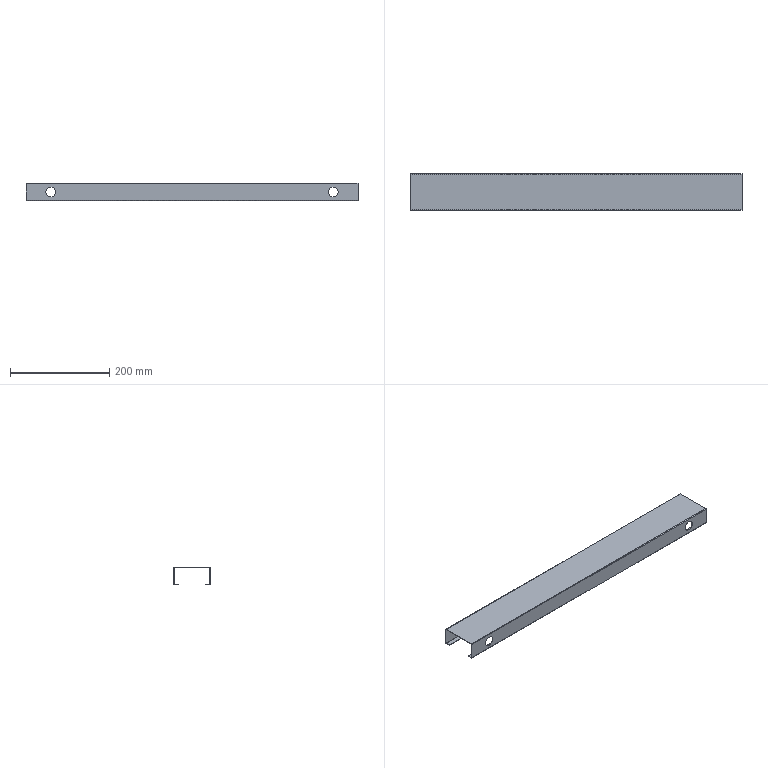Part | SolidWorks | features Cut 2, EdgeFlange 2, FlatPattern 1, ICE 1, SMBaseFlange 1, SheetMetal 1 | 1 solid | 58 faces | box 668 x 74 x 35 mm | volume 99136 mm3 | plane 40 | cylinder 18 | commonest cylinder face diameters 20 x8 0.4 x5 2.4 x5
STEP:
#1=CARTESIAN_POINT('',(-284.,36.,-27.5));
#2=VERTEX_POINT('',#1);
#3=CARTESIAN_POINT('',(-284.,36.,-7.5));
#4=VERTEX_POINT('',#3);
#5=CARTESIAN_POINT('',(-284.,36.,-17.5));
#6=DIRECTION('',(0.,1.,0.));
#7=DIRECTION('',(0.,0.,1.));
#8=AXIS2_PLACEMENT_3D('',#5,#6,#7);
#9=CIRCLE('',#8,10.);
#10=EDGE_CURVE('',#2,#4,#9,.T.);
#11=ORIENTED_EDGE('',*,*,#10,.F.);
#12=CARTESIAN_POINT('',(-284.,37.,-27.5));
#13=VERTEX_POINT('',#12);
#14=CARTESIAN_POINT('',(-284.,-37.,-27.5));
#15=DIRECTION('',(0.,1.,0.));
#16=VECTOR('',#15,1000.);
#17=LINE('',#14,#16);
#18=EDGE_CURVE('',#2,#13,#17,.T.);
#19=ORIENTED_EDGE('',*,*,#18,.T.);
#20=CARTESIAN_POINT('',(-284.,37.,-7.5));
#21=VERTEX_POINT('',#20);
#22=CARTESIAN_POINT('',(-284.,37.,-17.5));
#23=DIRECTION('',(0.,1.,0.));
#24=DIRECTION('',(0.,0.,1.));
#25=AXIS2_PLACEMENT_3D('',#22,#23,#24);
#26=CIRCLE('',#25,10.);
#27=EDGE_CURVE('',#13,#21,#26,.T.);
#28=ORIENTED_EDGE('',*,*,#27,.T.);
#29=CARTESIAN_POINT('',(-284.,-37.,-7.5));
#30=DIRECTION('',(0.,1.,0.));
#31=VECTOR('',#30,1000.);
#32=LINE('',#29,#31);
#33=EDGE_CURVE('',#4,#21,#32,.T.);
#34=ORIENTED_EDGE('',*,*,#33,.F.);
#35=EDGE_LOOP('',(#11,#19,#28,#34));
#36=FACE_OUTER_BOUND('',#35,.T.);
#37=CARTESIAN_POINT('',(-284.,-37.,-17.5));
#38=DIRECTION('',(0.,1.,0.));
#39=DIRECTION('',(0.,0.,1.));
#40=AXIS2_PLACEMENT_3D('',#37,#38,#39);
#41=CYLINDRICAL_SURFACE('',#40,10.);
#42=ADVANCED_FACE('',(#36),#41,.F.);
#43=CARTESIAN_POINT('',(284.,36.,-27.5));
#44=VERTEX_POINT('',#43);
#45=CARTESIAN_POINT('',(284.,36.,-7.5));
#46=VERTEX_POINT('',#45);
#47=CARTESIAN_POINT('',(284.,36.,-17.5));
#48=DIRECTION('',(0.,1.,0.));
#49=DIRECTION('',(0.,0.,1.));
#50=AXIS2_PLACEMENT_3D('',#47,#48,#49);
#51=CIRCLE('',#50,10.);
#52=EDGE_CURVE('',#44,#46,#51,.T.);
#53=ORIENTED_EDGE('',*,*,#52,.F.);
#54=CARTESIAN_POINT('',(284.,37.,-27.5));
#55=VERTEX_POINT('',#54);
#56=CARTESIAN_POINT('',(284.,-37.,-27.5));
#57=DIRECTION('',(0.,1.,0.));
#58=VECTOR('',#57,1000.);
#59=LINE('',#56,#58);
#60=EDGE_CURVE('',#44,#55,#59,.T.);
#61=ORIENTED_EDGE('',*,*,#60,.T.);
#62=CARTESIAN_POINT('',(284.,37.,-7.5));
#63=VERTEX_POINT('',#62);
#64=CARTESIAN_POINT('',(284.,37.,-17.5));
#65=DIRECTION('',(0.,1.,0.));
#66=DIRECTION('',(0.,0.,1.));
#67=AXIS2_PLACEMENT_3D('',#64,#65,#66);
#68=CIRCLE('',#67,10.);
#69=EDGE_CURVE('',#55,#63,#68,.T.);
#70=ORIENTED_EDGE('',*,*,#69,.T.);
#71=CARTESIAN_POINT('',(284.,-37.,-7.5));
#72=DIRECTION('',(0.,1.,0.));
#73=VECTOR('',#72,1000.);
#74=LINE('',#71,#73);
#75=EDGE_CURVE('',#46,#63,#74,.T.);
#76=ORIENTED_EDGE('',*,*,#75,.F.);
#77=EDGE_LOOP('',(#53,#61,#70,#76));
#78=FACE_OUTER_BOUND('',#77,.T.);
#79=CARTESIAN_POINT('',(284.,-37.,-17.5));
#80=DIRECTION('',(0.,1.,0.));
#81=DIRECTION('',(0.,0.,1.));
#82=AXIS2_PLACEMENT_3D('',#79,#80,#81);
#83=CYLINDRICAL_SURFACE('',#82,10.);
#84=ADVANCED_FACE('',(#78),#83,.F.);
#85=CARTESIAN_POINT('',(-284.,-37.,-27.5));
#86=VERTEX_POINT('',#85);
#87=CARTESIAN_POINT('',(-284.,-37.,-7.5));
#88=VERTEX_POINT('',#87);
#89=CARTESIAN_POINT('',(-284.,-37.,-17.5));
#90=DIRECTION('',(0.,1.,0.));
#91=DIRECTION('',(0.,0.,1.));
#92=AXIS2_PLACEMENT_3D('',#89,#90,#91);
#93=CIRCLE('',#92,10.);
#94=EDGE_CURVE('',#86,#88,#93,.T.);
#95=ORIENTED_EDGE('',*,*,#94,.F.);
#96=CARTESIAN_POINT('',(-284.,-36.,-27.5));
#97=VERTEX_POINT('',#96);
#98=CARTESIAN_POINT('',(-284.,-37.,-27.5));
#99=DIRECTION('',(0.,1.,0.));
#100=VECTOR('',#99,1000.);
#101=LINE('',#98,#100);
#102=EDGE_CURVE('',#86,#97,#101,.T.);
#103=ORIENTED_EDGE('',*,*,#102,.T.);
#104=CARTESIAN_POINT('',(-284.,-36.,-7.5));
#105=VERTEX_POINT('',#104);
#106=CARTESIAN_POINT('',(-284.,-36.,-17.5));
#107=DIRECTION('',(0.,1.,0.));
#108=DIRECTION('',(0.,0.,1.));
#109=AXIS2_PLACEMENT_3D('',#106,#107,#108);
#110=CIRCLE('',#109,10.);
#111=EDGE_CURVE('',#97,#105,#110,.T.);
#112=ORIENTED_EDGE('',*,*,#111,.T.);
#113=CARTESIAN_POINT('',(-284.,-37.,-7.5));
#114=DIRECTION('',(0.,1.,0.));
#115=VECTOR('',#114,1000.);
#116=LINE('',#113,#115);
#117=EDGE_CURVE('',#88,#105,#116,.T.);
#118=ORIENTED_EDGE('',*,*,#117,.F.);
#119=EDGE_LOOP('',(#95,#103,#112,#118));
#120=FACE_OUTER_BOUND('',#119,.T.);
#121=CARTESIAN_POINT('',(-284.,-37.,-17.5));
#122=DIRECTION('',(0.,1.,0.));
#123=DIRECTION('',(0.,0.,1.));
#124=AXIS2_PLACEMENT_3D('',#121,#122,#123);
#125=CYLINDRICAL_SURFACE('',#124,10.);
#126=ADVANCED_FACE('',(#120),#125,.F.);
#127=CARTESIAN_POINT('',(284.,-37.,-27.5));
#128=VERTEX_POINT('',#127);
#129=CARTESIAN_POINT('',(284.,-37.,-7.5));
#130=VERTEX_POINT('',#129);
#131=CARTESIAN_POINT('',(284.,-37.,-17.5));
#132=DIRECTION('',(0.,1.,0.));
#133=DIRECTION('',(0.,0.,-1.));
#134=AXIS2_PLACEMENT_3D('',#131,#132,#133);
#135=CIRCLE('',#134,10.);
#136=EDGE_CURVE('',#128,#130,#135,.T.);
#137=ORIENTED_EDGE('',*,*,#136,.F.);
#138=CARTESIAN_POINT('',(284.,-36.,-27.5));
#139=VERTEX_POINT('',#138);
#140=CARTESIAN_POINT('',(284.,-37.,-27.5));
#141=DIRECTION('',(0.,1.,0.));
#142=VECTOR('',#141,1000.);
#143=LINE('',#140,#142);
#144=EDGE_CURVE('',#128,#139,#143,.T.);
#145=ORIENTED_EDGE('',*,*,#144,.T.);
#146=CARTESIAN_POINT('',(284.,-36.,-7.5));
#147=VERTEX_POINT('',#146);
#148=CARTESIAN_POINT('',(284.,-36.,-17.5));
#149=DIRECTION('',(0.,1.,0.));
#150=DIRECTION('',(0.,0.,1.));
#151=AXIS2_PLACEMENT_3D('',#148,#149,#150);
#152=CIRCLE('',#151,10.);
#153=EDGE_CURVE('',#139,#147,#152,.T.);
#154=ORIENTED_EDGE('',*,*,#153,.T.);
#155=CARTESIAN_POINT('',(284.,-37.,-7.5));
#156=DIRECTION('',(0.,1.,0.));
#157=VECTOR('',#156,1000.);
#158=LINE('',#155,#157);
#159=EDGE_CURVE('',#130,#147,#158,.T.);
#160=ORIENTED_EDGE('',*,*,#159,.F.);
#161=EDGE_LOOP('',(#137,#145,#154,#160));
#162=FACE_OUTER_BOUND('',#161,.T.);
#163=CARTESIAN_POINT('',(284.,-37.,-17.5));
#164=DIRECTION('',(0.,1.,0.));
#165=DIRECTION('',(0.,0.,1.));
#166=AXIS2_PLACEMENT_3D('',#163,#164,#165);
#167=CYLINDRICAL_SURFACE('',#166,10.);
#168=ADVANCED_FACE('',(#162),#167,.F.);
#169=CARTESIAN_POINT('',(-152.,27.,-35.));
#170=VERTEX_POINT('',#169);
#171=CARTESIAN_POINT('',(-152.,35.8,-35.));
#172=VERTEX_POINT('',#171);
#173=CARTESIAN_POINT('',(-152.,47.,-35.));
#174=DIRECTION('',(0.,1.,0.));
#175=VECTOR('',#174,1000.);
#176=LINE('',#173,#175);
#177=EDGE_CURVE('',#170,#172,#176,.T.);
#178=ORIENTED_EDGE('',*,*,#177,.T.);
#179=CARTESIAN_POINT('',(-152.,35.8,-34.));
#180=VERTEX_POINT('',#179);
#181=CARTESIAN_POINT('',(-152.,35.8,-35.));
#182=DIRECTION('',(0.,0.,1.));
#183=VECTOR('',#182,1000.);
#184=LINE('',#181,#183);
#185=EDGE_CURVE('',#172,#180,#184,.T.);
#186=ORIENTED_EDGE('',*,*,#185,.T.);
#187=CARTESIAN_POINT('',(-152.,27.,-34.));
#188=VERTEX_POINT('',#187);
#189=CARTESIAN_POINT('',(-152.,0.,-34.));
#190=DIRECTION('',(0.,-1.,0.));
#191=VECTOR('',#190,1000.);
#192=LINE('',#189,#191);
#193=EDGE_CURVE('',#180,#188,#192,.T.);
#194=ORIENTED_EDGE('',*,*,#193,.T.);
#195=CARTESIAN_POINT('',(-152.,27.,-35.));
#196=DIRECTION('',(0.,0.,1.));
#197=VECTOR('',#196,1000.);
#198=LINE('',#195,#197);
#199=EDGE_CURVE('',#170,#188,#198,.T.);
#200=ORIENTED_EDGE('',*,*,#199,.F.);
#201=EDGE_LOOP('',(#178,#186,#194,#200));
#202=FACE_OUTER_BOUND('',#201,.T.);
#203=CARTESIAN_POINT('',(-152.,47.,-25.));
#204=DIRECTION('',(-1.,0.,0.));
#205=DIRECTION('',(0.,0.,1.));
#206=AXIS2_PLACEMENT_3D('',#203,#204,#205);
#207=PLANE('',#206);
#208=ADVANCED_FACE('',(#202),#207,.F.);
#209=CARTESIAN_POINT('',(-152.,36.,-33.8));
#210=VERTEX_POINT('',#209);
#211=CARTESIAN_POINT('',(-152.,36.,-25.));
#212=VERTEX_POINT('',#211);
#213=CARTESIAN_POINT('',(-152.,36.,0.));
#214=DIRECTION('',(0.,0.,1.));
#215=VECTOR('',#214,1000.);
#216=LINE('',#213,#215);
#217=EDGE_CURVE('',#210,#212,#216,.T.);
#218=ORIENTED_EDGE('',*,*,#217,.F.);
#219=CARTESIAN_POINT('',(-152.,37.,-33.8));
#220=VERTEX_POINT('',#219);
#221=CARTESIAN_POINT('',(-152.,36.,-33.8));
#222=DIRECTION('',(0.,1.,0.));
#223=VECTOR('',#222,1000.);
#224=LINE('',#221,#223);
#225=EDGE_CURVE('',#210,#220,#224,.T.);
#226=ORIENTED_EDGE('',*,*,#225,.T.);
#227=CARTESIAN_POINT('',(-152.,37.,-25.));
#228=VERTEX_POINT('',#227);
#229=CARTESIAN_POINT('',(-152.,37.,0.));
#230=DIRECTION('',(0.,0.,1.));
#231=VECTOR('',#230,1000.);
#232=LINE('',#229,#231);
#233=EDGE_CURVE('',#220,#228,#232,.T.);
#234=ORIENTED_EDGE('',*,*,#233,.T.);
#235=CARTESIAN_POINT('',(-152.,47.,-25.));
#236=DIRECTION('',(0.,1.,0.));
#237=VECTOR('',#236,1000.);
#238=LINE('',#235,#237);
#239=EDGE_CURVE('',#212,#228,#238,.T.);
#240=ORIENTED_EDGE('',*,*,#239,.F.);
#241=EDGE_LOOP('',(#218,#226,#234,#240));
#242=FACE_OUTER_BOUND('',#241,.T.);
#243=CARTESIAN_POINT('',(-152.,47.,-25.));
#244=DIRECTION('',(-1.,0.,0.));
#245=DIRECTION('',(0.,0.,1.));
#246=AXIS2_PLACEMENT_3D('',#243,#244,#245);
#247=PLANE('',#246);
#248=ADVANCED_FACE('',(#242),#247,.F.);
#249=CARTESIAN_POINT('',(152.,27.,-34.));
#250=VERTEX_POINT('',#249);
#251=CARTESIAN_POINT('',(152.,35.8,-34.));
#252=VERTEX_POINT('',#251);
#253=CARTESIAN_POINT('',(152.,0.,-34.));
#254=DIRECTION('',(0.,1.,0.));
#255=VECTOR('',#254,1000.);
#256=LINE('',#253,#255);
#257=EDGE_CURVE('',#250,#252,#256,.T.);
#258=ORIENTED_EDGE('',*,*,#257,.T.);
#259=CARTESIAN_POINT('',(152.,35.8,-35.));
#260=VERTEX_POINT('',#259);
#261=CARTESIAN_POINT('',(152.,35.8,-34.));
#262=DIRECTION('',(0.,0.,-1.));
#263=VECTOR('',#262,1000.);
#264=LINE('',#261,#263);
#265=EDGE_CURVE('',#252,#260,#264,.T.);
#266=ORIENTED_EDGE('',*,*,#265,.T.);
#267=CARTESIAN_POINT('',(152.,27.,-35.));
#268=VERTEX_POINT('',#267);
#269=CARTESIAN_POINT('',(152.,47.,-35.));
#270=DIRECTION('',(0.,-1.,0.));
#271=VECTOR('',#270,1000.);
#272=LINE('',#269,#271);
#273=EDGE_CURVE('',#260,#268,#272,.T.);
#274=ORIENTED_EDGE('',*,*,#273,.T.);
#275=CARTESIAN_POINT('',(152.,27.,-35.));
#276=DIRECTION('',(0.,0.,-1.));
#277=VECTOR('',#276,1000.);
#278=LINE('',#275,#277);
#279=EDGE_CURVE('',#250,#268,#278,.T.);
#280=ORIENTED_EDGE('',*,*,#279,.F.);
#281=EDGE_LOOP('',(#258,#266,#274,#280));
#282=FACE_OUTER_BOUND('',#281,.T.);
#283=CARTESIAN_POINT('',(152.,47.,-25.));
#284=DIRECTION('',(1.,0.,0.));
#285=DIRECTION('',(0.,0.,-1.));
#286=AXIS2_PLACEMENT_3D('',#283,#284,#285);
#287=PLANE('',#286);
#288=ADVANCED_FACE('',(#282),#287,.F.);
#289=CARTESIAN_POINT('',(152.,37.,-25.));
#290=VERTEX_POINT('',#289);
#291=CARTESIAN_POINT('',(152.,37.,-33.8));
#292=VERTEX_POINT('',#291);
#293=CARTESIAN_POINT('',(152.,37.,0.));
#294=DIRECTION('',(0.,0.,-1.));
#295=VECTOR('',#294,1000.);
#296=LINE('',#293,#295);
#297=EDGE_CURVE('',#290,#292,#296,.T.);
#298=ORIENTED_EDGE('',*,*,#297,.T.);
#299=CARTESIAN_POINT('',(152.,36.,-33.8));
#300=VERTEX_POINT('',#299);
#301=CARTESIAN_POINT('',(152.,37.,-33.8));
#302=DIRECTION('',(0.,-1.,0.));
#303=VECTOR('',#302,1000.);
#304=LINE('',#301,#303);
#305=EDGE_CURVE('',#292,#300,#304,.T.);
#306=ORIENTED_EDGE('',*,*,#305,.T.);
#307=CARTESIAN_POINT('',(152.,36.,-25.));
#308=VERTEX_POINT('',#307);
#309=CARTESIAN_POINT('',(152.,36.,0.));
#310=DIRECTION('',(0.,0.,-1.));
#311=VECTOR('',#310,1000.);
#312=LINE('',#309,#311);
#313=EDGE_CURVE('',#308,#300,#312,.T.);
#314=ORIENTED_EDGE('',*,*,#313,.F.);
#315=CARTESIAN_POINT('',(152.,47.,-25.));
#316=DIRECTION('',(0.,-1.,0.));
#317=VECTOR('',#316,1000.);
#318=LINE('',#315,#317);
#319=EDGE_CURVE('',#290,#308,#318,.T.);
#320=ORIENTED_EDGE('',*,*,#319,.F.);
#321=EDGE_LOOP('',(#298,#306,#314,#320));
#322=FACE_OUTER_BOUND('',#321,.T.);
#323=CARTESIAN_POINT('',(152.,47.,-25.));
#324=DIRECTION('',(1.,0.,0.));
#325=DIRECTION('',(0.,0.,-1.));
#326=AXIS2_PLACEMENT_3D('',#323,#324,#325);
#327=PLANE('',#326);
#328=ADVANCED_FACE('',(#322),#327,.F.);
#329=CARTESIAN_POINT('',(152.,35.8,-33.8));
#330=DIRECTION('',(-1.,0.,0.));
#331=DIRECTION('',(0.,0.,-1.));
#332=AXIS2_PLACEMENT_3D('',#329,#330,#331);
#333=CIRCLE('',#332,1.2);
#334=EDGE_CURVE('',#292,#260,#333,.T.);
#335=ORIENTED_EDGE('',*,*,#334,.F.);
#336=CARTESIAN_POINT('',(334.,37.,-33.8));
#337=VERTEX_POINT('',#336);
#338=CARTESIAN_POINT('',(334.,37.,-33.8));
#339=DIRECTION('',(-1.,0.,0.));
#340=VECTOR('',#339,1000.);
#341=LINE('',#338,#340);
#342=EDGE_CURVE('',#337,#292,#341,.T.);
#343=ORIENTED_EDGE('',*,*,#342,.F.);
#344=CARTESIAN_POINT('',(334.,35.8,-35.));
#345=VERTEX_POINT('',#344);
#346=CARTESIAN_POINT('',(334.,35.8,-33.8));
#347=DIRECTION('',(1.,0.,0.));
#348=DIRECTION('',(0.,0.,-1.));
#349=AXIS2_PLACEMENT_3D('',#346,#347,#348);
#350=CIRCLE('',#349,1.2);
#351=EDGE_CURVE('',#345,#337,#350,.T.);
#352=ORIENTED_EDGE('',*,*,#351,.F.);
#353=CARTESIAN_POINT('',(-334.,35.8,-35.));
#354=DIRECTION('',(-1.,0.,0.));
#355=VECTOR('',#354,1000.);
#356=LINE('',#353,#355);
#357=EDGE_CURVE('',#345,#260,#356,.T.);
#358=ORIENTED_EDGE('',*,*,#357,.T.);
#359=EDGE_LOOP('',(#335,#343,#352,#358));
#360=FACE_OUTER_BOUND('',#359,.T.);
#361=CARTESIAN_POINT('',(334.,35.8,-33.8));
#362=DIRECTION('',(1.,0.,0.));
#363=DIRECTION('',(0.,0.,-1.));
#364=AXIS2_PLACEMENT_3D('',#361,#362,#363);
#365=CYLINDRICAL_SURFACE('',#364,1.2);
#366=ADVANCED_FACE('',(#360),#365,.T.);
#367=CARTESIAN_POINT('',(334.,36.,-33.8));
#368=VERTEX_POINT('',#367);
#369=CARTESIAN_POINT('',(334.,36.,-33.8));
#370=DIRECTION('',(-1.,0.,0.));
#371=VECTOR('',#370,1000.);
#372=LINE('',#369,#371);
#373=EDGE_CURVE('',#368,#300,#372,.T.);
#374=ORIENTED_EDGE('',*,*,#373,.T.);
#375=CARTESIAN_POINT('',(152.,35.8,-33.8));
#376=DIRECTION('',(-1.,0.,0.));
#377=DIRECTION('',(0.,0.,-1.));
#378=AXIS2_PLACEMENT_3D('',#375,#376,#377);
#379=CIRCLE('',#378,0.2);
#380=EDGE_CURVE('',#300,#252,#379,.T.);
#381=ORIENTED_EDGE('',*,*,#380,.T.);
#382=CARTESIAN_POINT('',(334.,35.8,-34.));
#383=VERTEX_POINT('',#382);
#384=CARTESIAN_POINT('',(-334.,35.8,-34.));
#385=DIRECTION('',(1.,0.,0.));
#386=VECTOR('',#385,1000.);
#387=LINE('',#384,#386);
#388=EDGE_CURVE('',#252,#383,#387,.T.);
#389=ORIENTED_EDGE('',*,*,#388,.T.);
#390=CARTESIAN_POINT('',(334.,35.8,-33.8));
#391=DIRECTION('',(1.,0.,0.));
#392=DIRECTION('',(0.,0.,-1.));
#393=AXIS2_PLACEMENT_3D('',#390,#391,#392);
#394=CIRCLE('',#393,0.2);
#395=EDGE_CURVE('',#383,#368,#394,.T.);
#396=ORIENTED_EDGE('',*,*,#395,.T.);
#397=EDGE_LOOP('',(#374,#381,#389,#396));
#398=FACE_OUTER_BOUND('',#397,.T.);
#399=CARTESIAN_POINT('',(334.,35.8,-33.8));
#400=DIRECTION('',(1.,0.,0.));
#401=DIRECTION('',(0.,0.,-1.));
#402=AXIS2_PLACEMENT_3D('',#399,#400,#401);
#403=CYLINDRICAL_SURFACE('',#402,0.2);
#404=ADVANCED_FACE('',(#398),#403,.F.);
#405=CARTESIAN_POINT('',(334.,27.,-35.));
#406=VERTEX_POINT('',#405);
#407=CARTESIAN_POINT('',(0.,27.,-35.));
#408=DIRECTION('',(-1.,0.,0.));
#409=VECTOR('',#408,1000.);
#410=LINE('',#407,#409);
#411=EDGE_CURVE('',#406,#268,#410,.T.);
#412=ORIENTED_EDGE('',*,*,#411,.T.);
#413=ORIENTED_EDGE('',*,*,#273,.F.);
#414=ORIENTED_EDGE('',*,*,#357,.F.);
#415=CARTESIAN_POINT('',(334.,0.,-35.));
#416=DIRECTION('',(0.,-1.,0.));
#417=VECTOR('',#416,1000.);
#418=LINE('',#415,#417);
#419=EDGE_CURVE('',#345,#406,#418,.T.);
#420=ORIENTED_EDGE('',*,*,#419,.T.);
#421=EDGE_LOOP('',(#412,#413,#414,#420));
#422=FACE_OUTER_BOUND('',#421,.T.);
#423=CARTESIAN_POINT('',(0.,0.,-35.));
#424=DIRECTION('',(0.,0.,1.));
#425=DIRECTION('',(0.,-1.,0.));
#426=AXIS2_PLACEMENT_3D('',#423,#424,#425);
#427=PLANE('',#426);
#428=ADVANCED_FACE('',(#422),#427,.F.);
#429=ORIENTED_EDGE('',*,*,#257,.F.);
#430=CARTESIAN_POINT('',(334.,27.,-34.));
#431=VERTEX_POINT('',#430);
#432=CARTESIAN_POINT('',(-334.,27.,-34.));
#433=DIRECTION('',(-1.,0.,0.));
#434=VECTOR('',#433,1000.);
#435=LINE('',#432,#434);
#436=EDGE_CURVE('',#431,#250,#435,.T.);
#437=ORIENTED_EDGE('',*,*,#436,.F.);
#438=CARTESIAN_POINT('',(334.,27.,-34.));
#439=DIRECTION('',(0.,-1.,0.));
#440=VECTOR('',#439,1000.);
#441=LINE('',#438,#440);
#442=EDGE_CURVE('',#383,#431,#441,.T.);
#443=ORIENTED_EDGE('',*,*,#442,.F.);
#444=ORIENTED_EDGE('',*,*,#388,.F.);
#445=EDGE_LOOP('',(#429,#437,#443,#444));
#446=FACE_OUTER_BOUND('',#445,.T.);
#447=CARTESIAN_POINT('',(0.,0.,-34.));
#448=DIRECTION('',(0.,0.,1.));
#449=DIRECTION('',(0.,-1.,0.));
#450=AXIS2_PLACEMENT_3D('',#447,#448,#449);
#451=PLANE('',#450);
#452=ADVANCED_FACE('',(#446),#451,.T.);
#453=ORIENTED_EDGE('',*,*,#436,.T.);
#454=ORIENTED_EDGE('',*,*,#279,.T.);
#455=ORIENTED_EDGE('',*,*,#411,.F.);
#456=CARTESIAN_POINT('',(334.,27.,-35.));
#457=DIRECTION('',(0.,0.,1.));
#458=VECTOR('',#457,1000.);
#459=LINE('',#456,#458);
#460=EDGE_CURVE('',#406,#431,#459,.T.);
#461=ORIENTED_EDGE('',*,*,#460,.T.);
#462=EDGE_LOOP('',(#453,#454,#455,#461));
#463=FACE_OUTER_BOUND('',#462,.T.);
#464=CARTESIAN_POINT('',(-334.,27.,-35.));
#465=DIRECTION('',(0.,1.,0.));
#466=DIRECTION('',(0.,0.,1.));
#467=AXIS2_PLACEMENT_3D('',#464,#465,#466);
#468=PLANE('',#467);
#469=ADVANCED_FACE('',(#463),#468,.F.);
#470=CARTESIAN_POINT('',(334.,36.,-1.2));
#471=VERTEX_POINT('',#470);
#472=CARTESIAN_POINT('',(334.,36.,0.));
#473=DIRECTION('',(0.,0.,1.));
#474=VECTOR('',#473,1000.);
#475=LINE('',#472,#474);
#476=EDGE_CURVE('',#368,#471,#475,.T.);
#477=ORIENTED_EDGE('',*,*,#476,.F.);
#478=CARTESIAN_POINT('',(334.,36.,-33.8));
#479=DIRECTION('',(0.,1.,0.));
#480=VECTOR('',#479,1000.);
#481=LINE('',#478,#480);
#482=EDGE_CURVE('',#368,#337,#481,.T.);
#483=ORIENTED_EDGE('',*,*,#482,.T.);
#484=CARTESIAN_POINT('',(334.,37.,-1.2));
#485=VERTEX_POINT('',#484);
#486=CARTESIAN_POINT('',(334.,37.,-1.));
#487=DIRECTION('',(0.,0.,1.));
#488=VECTOR('',#487,1000.);
#489=LINE('',#486,#488);
#490=EDGE_CURVE('',#337,#485,#489,.T.);
#491=ORIENTED_EDGE('',*,*,#490,.T.);
#492=CARTESIAN_POINT('',(334.,36.,-1.2));
#493=DIRECTION('',(0.,1.,0.));
#494=VECTOR('',#493,1000.);
#495=LINE('',#492,#494);
#496=EDGE_CURVE('',#471,#485,#495,.T.);
#497=ORIENTED_EDGE('',*,*,#496,.F.);
#498=EDGE_LOOP('',(#477,#483,#491,#497));
#499=FACE_OUTER_BOUND('',#498,.T.);
#500=CARTESIAN_POINT('',(334.,37.,-1.));
#501=DIRECTION('',(1.,0.,0.));
#502=DIRECTION('',(0.,0.,-1.));
#503=AXIS2_PLACEMENT_3D('',#500,#501,#502);
#504=PLANE('',#503);
#505=ADVANCED_FACE('',(#499),#504,.T.);
#506=ORIENTED_EDGE('',*,*,#297,.F.);
#507=CARTESIAN_POINT('',(0.,37.,-25.));
#508=DIRECTION('',(1.,0.,0.));
#509=VECTOR('',#508,1000.);
#510=LINE('',#507,#509);
#511=EDGE_CURVE('',#228,#290,#510,.T.);
#512=ORIENTED_EDGE('',*,*,#511,.F.);
#513=ORIENTED_EDGE('',*,*,#233,.F.);
#514=CARTESIAN_POINT('',(-334.,37.,-33.8));
#515=VERTEX_POINT('',#514);
#516=CARTESIAN_POINT('',(334.,37.,-33.8));
#517=DIRECTION('',(-1.,0.,0.));
#518=VECTOR('',#517,1000.);
#519=LINE('',#516,#518);
#520=EDGE_CURVE('',#220,#515,#519,.T.);
#521=ORIENTED_EDGE('',*,*,#520,.T.);
#522=CARTESIAN_POINT('',(-334.,37.,-1.2));
#523=VERTEX_POINT('',#522);
#524=CARTESIAN_POINT('',(-334.,37.,-35.));
#525=DIRECTION('',(0.,0.,-1.));
#526=VECTOR('',#525,1000.);
#527=LINE('',#524,#526);
#528=EDGE_CURVE('',#523,#515,#527,.T.);
#529=ORIENTED_EDGE('',*,*,#528,.F.);
#530=CARTESIAN_POINT('',(0.,37.,-1.2));
#531=DIRECTION('',(1.,0.,0.));
#532=VECTOR('',#531,1000.);
#533=LINE('',#530,#532);
#534=EDGE_CURVE('',#523,#485,#533,.T.);
#535=ORIENTED_EDGE('',*,*,#534,.T.);
#536=ORIENTED_EDGE('',*,*,#490,.F.);
#537=ORIENTED_EDGE('',*,*,#342,.T.);
#538=EDGE_LOOP('',(#506,#512,#513,#521,#529,#535,#536,#537));
#539=FACE_OUTER_BOUND('',#538,.T.);
#540=CARTESIAN_POINT('',(-284.,37.,-17.5));
#541=DIRECTION('',(0.,1.,0.));
#542=DIRECTION('',(0.,0.,1.));
#543=AXIS2_PLACEMENT_3D('',#540,#541,#542);
#544=CIRCLE('',#543,10.);
#545=EDGE_CURVE('',#21,#13,#544,.T.);
#546=ORIENTED_EDGE('',*,*,#545,.F.);
#547=ORIENTED_EDGE('',*,*,#27,.F.);
#548=EDGE_LOOP('',(#546,#547));
#549=FACE_BOUND('',#548,.T.);
#550=CARTESIAN_POINT('',(284.,37.,-17.5));
#551=DIRECTION('',(0.,1.,0.));
#552=DIRECTION('',(0.,0.,1.));
#553=AXIS2_PLACEMENT_3D('',#550,#551,#552);
#554=CIRCLE('',#553,10.);
#555=EDGE_CURVE('',#63,#55,#554,.T.);
#556=ORIENTED_EDGE('',*,*,#555,.F.);
#557=ORIENTED_EDGE('',*,*,#69,.F.);
#558=EDGE_LOOP('',(#556,#557));
#559=FACE_BOUND('',#558,.T.);
#560=CARTESIAN_POINT('',(0.,37.,0.));
#561=DIRECTION('',(0.,1.,0.));
#562=DIRECTION('',(0.,0.,1.));
#563=AXIS2_PLACEMENT_3D('',#560,#561,#562);
#564=PLANE('',#563);
#565=ADVANCED_FACE('',(#539,#549,#559),#564,.T.);
#566=CARTESIAN_POINT('',(-284.,36.,-17.5));
#567=DIRECTION('',(0.,1.,0.));
#568=DIRECTION('',(0.,0.,1.));
#569=AXIS2_PLACEMENT_3D('',#566,#567,#568);
#570=CIRCLE('',#569,10.);
#571=EDGE_CURVE('',#4,#2,#570,.T.);
#572=ORIENTED_EDGE('',*,*,#571,.T.);
#573=ORIENTED_EDGE('',*,*,#10,.T.);
#574=EDGE_LOOP('',(#572,#573));
#575=FACE_BOUND('',#574,.T.);
#576=CARTESIAN_POINT('',(284.,36.,-17.5));
#577=DIRECTION('',(0.,1.,0.));
#578=DIRECTION('',(0.,0.,1.));
#579=AXIS2_PLACEMENT_3D('',#576,#577,#578);
#580=CIRCLE('',#579,10.);
#581=EDGE_CURVE('',#46,#44,#580,.T.);
#582=ORIENTED_EDGE('',*,*,#581,.T.);
#583=ORIENTED_EDGE('',*,*,#52,.T.);
#584=EDGE_LOOP('',(#582,#583));
#585=FACE_BOUND('',#584,.T.);
#586=CARTESIAN_POINT('',(0.,36.,-25.));
#587=DIRECTION('',(1.,0.,0.));
#588=VECTOR('',#587,1000.);
#589=LINE('',#586,#588);
#590=EDGE_CURVE('',#212,#308,#589,.T.);
#591=ORIENTED_EDGE('',*,*,#590,.T.);
#592=ORIENTED_EDGE('',*,*,#313,.T.);
#593=ORIENTED_EDGE('',*,*,#373,.F.);
#594=ORIENTED_EDGE('',*,*,#476,.T.);
#595=CARTESIAN_POINT('',(-334.,36.,-1.2));
#596=VERTEX_POINT('',#595);
#597=CARTESIAN_POINT('',(-334.,36.,-1.2));
#598=DIRECTION('',(1.,0.,0.));
#599=VECTOR('',#598,1000.);
#600=LINE('',#597,#599);
#601=EDGE_CURVE('',#596,#471,#600,.T.);
#602=ORIENTED_EDGE('',*,*,#601,.F.);
#603=CARTESIAN_POINT('',(-334.,36.,-33.8));
#604=VERTEX_POINT('',#603);
#605=CARTESIAN_POINT('',(-334.,36.,0.));
#606=DIRECTION('',(0.,0.,-1.));
#607=VECTOR('',#606,1000.);
#608=LINE('',#605,#607);
#609=EDGE_CURVE('',#596,#604,#608,.T.);
#610=ORIENTED_EDGE('',*,*,#609,.T.);
#611=CARTESIAN_POINT('',(334.,36.,-33.8));
#612=DIRECTION('',(-1.,0.,0.));
#613=VECTOR('',#612,1000.);
#614=LINE('',#611,#613);
#615=EDGE_CURVE('',#210,#604,#614,.T.);
#616=ORIENTED_EDGE('',*,*,#615,.F.);
#617=ORIENTED_EDGE('',*,*,#217,.T.);
#618=EDGE_LOOP('',(#591,#592,#593,#594,#602,#610,#616,#617));
#619=FACE_OUTER_BOUND('',#618,.T.);
#620=CARTESIAN_POINT('',(0.,36.,0.));
#621=DIRECTION('',(0.,1.,0.));
#622=DIRECTION('',(0.,0.,1.));
#623=AXIS2_PLACEMENT_3D('',#620,#621,#622);
#624=PLANE('',#623);
#625=ADVANCED_FACE('',(#575,#585,#619),#624,.F.);
#626=CARTESIAN_POINT('',(-334.,-36.,-33.8));
#627=VERTEX_POINT('',#626);
#628=CARTESIAN_POINT('',(-334.,-36.,-1.2));
#629=VERTEX_POINT('',#628);
#630=CARTESIAN_POINT('',(-334.,-36.,0.));
#631=DIRECTION('',(0.,0.,1.));
#632=VECTOR('',#631,1000.);
#633=LINE('',#630,#632);
#634=EDGE_CURVE('',#627,#629,#633,.T.);
#635=ORIENTED_EDGE('',*,*,#634,.F.);
#636=CARTESIAN_POINT('',(-334.,-37.,-33.8));
#637=VERTEX_POINT('',#636);
#638=CARTESIAN_POINT('',(-334.,-36.,-33.8));
#639=DIRECTION('',(0.,-1.,0.));
#640=VECTOR('',#639,1000.);
#641=LINE('',#638,#640);
#642=EDGE_CURVE('',#627,#637,#641,.T.);
#643=ORIENTED_EDGE('',*,*,#642,.T.);
#644=CARTESIAN_POINT('',(-334.,-37.,-1.2));
#645=VERTEX_POINT('',#644);
#646=CARTESIAN_POINT('',(-334.,-37.,-35.));
#647=DIRECTION('',(0.,0.,1.));
#648=VECTOR('',#647,1000.);
#649=LINE('',#646,#648);
#650=EDGE_CURVE('',#637,#645,#649,.T.);
#651=ORIENTED_EDGE('',*,*,#650,.T.);
#652=CARTESIAN_POINT('',(-334.,-36.,-1.2));
#653=DIRECTION('',(0.,-1.,0.));
#654=VECTOR('',#653,1000.);
#655=LINE('',#652,#654);
#656=EDGE_CURVE('',#629,#645,#655,.T.);
#657=ORIENTED_EDGE('',*,*,#656,.F.);
#658=EDGE_LOOP('',(#635,#643,#651,#657));
#659=FACE_OUTER_BOUND('',#658,.T.);
#660=CARTESIAN_POINT('',(-334.,-37.,-35.));
#661=DIRECTION('',(-1.,0.,0.));
#662=DIRECTION('',(0.,0.,1.));
#663=AXIS2_PLACEMENT_3D('',#660,#661,#662);
#664=PLANE('',#663);
#665=ADVANCED_FACE('',(#659),#664,.T.);
#666=CARTESIAN_POINT('',(-284.,-37.,-17.5));
#667=DIRECTION('',(0.,1.,0.));
#668=DIRECTION('',(0.,0.,1.));
#669=AXIS2_PLACEMENT_3D('',#666,#667,#668);
#670=CIRCLE('',#669,10.);
#671=EDGE_CURVE('',#88,#86,#670,.T.);
#672=ORIENTED_EDGE('',*,*,#671,.T.);
#673=ORIENTED_EDGE('',*,*,#94,.T.);
#674=EDGE_LOOP('',(#672,#673));
#675=FACE_BOUND('',#674,.T.);
#676=CARTESIAN_POINT('',(284.,-37.,-17.5));
#677=DIRECTION('',(0.,1.,0.));
#678=DIRECTION('',(0.,0.,-1.));
#679=AXIS2_PLACEMENT_3D('',#676,#677,#678);
#680=CIRCLE('',#679,10.);
#681=EDGE_CURVE('',#130,#128,#680,.T.);
#682=ORIENTED_EDGE('',*,*,#681,.T.);
#683=ORIENTED_EDGE('',*,*,#136,.T.);
#684=EDGE_LOOP('',(#682,#683));
#685=FACE_BOUND('',#684,.T.);
#686=CARTESIAN_POINT('',(334.,-37.,-33.8));
#687=VERTEX_POINT('',#686);
#688=CARTESIAN_POINT('',(-334.,-37.,-33.8));
#689=DIRECTION('',(1.,0.,0.));
#690=VECTOR('',#689,1000.);
#691=LINE('',#688,#690);
#692=EDGE_CURVE('',#637,#687,#691,.T.);
#693=ORIENTED_EDGE('',*,*,#692,.T.);
#694=CARTESIAN_POINT('',(334.,-37.,-1.2));
#695=VERTEX_POINT('',#694);
#696=CARTESIAN_POINT('',(334.,-37.,-1.));
#697=DIRECTION('',(0.,0.,-1.));
#698=VECTOR('',#697,1000.);
#699=LINE('',#696,#698);
#700=EDGE_CURVE('',#695,#687,#699,.T.);
#701=ORIENTED_EDGE('',*,*,#700,.F.);
#702=CARTESIAN_POINT('',(334.,-37.,-1.2));
#703=DIRECTION('',(1.,0.,0.));
#704=VECTOR('',#703,1000.);
#705=LINE('',#702,#704);
#706=EDGE_CURVE('',#645,#695,#705,.T.);
#707=ORIENTED_EDGE('',*,*,#706,.F.);
#708=ORIENTED_EDGE('',*,*,#650,.F.);
#709=EDGE_LOOP('',(#693,#701,#707,#708));
#710=FACE_OUTER_BOUND('',#709,.T.);
#711=CARTESIAN_POINT('',(0.,-37.,0.));
#712=DIRECTION('',(0.,1.,0.));
#713=DIRECTION('',(0.,0.,1.));
#714=AXIS2_PLACEMENT_3D('',#711,#712,#713);
#715=PLANE('',#714);
#716=ADVANCED_FACE('',(#675,#685,#710),#715,.F.);
#717=CARTESIAN_POINT('',(-284.,-36.,-17.5));
#718=DIRECTION('',(0.,1.,0.));
#719=DIRECTION('',(0.,0.,1.));
#720=AXIS2_PLACEMENT_3D('',#717,#718,#719);
#721=CIRCLE('',#720,10.);
#722=EDGE_CURVE('',#105,#97,#721,.T.);
#723=ORIENTED_EDGE('',*,*,#722,.F.);
#724=ORIENTED_EDGE('',*,*,#111,.F.);
#725=EDGE_LOOP('',(#723,#724));
#726=FACE_BOUND('',#725,.T.);
#727=CARTESIAN_POINT('',(284.,-36.,-17.5));
#728=DIRECTION('',(0.,1.,0.));
#729=DIRECTION('',(0.,0.,1.));
#730=AXIS2_PLACEMENT_3D('',#727,#728,#729);
#731=CIRCLE('',#730,10.);
#732=EDGE_CURVE('',#147,#139,#731,.T.);
#733=ORIENTED_EDGE('',*,*,#732,.F.);
#734=ORIENTED_EDGE('',*,*,#153,.F.);
#735=EDGE_LOOP('',(#733,#734));
#736=FACE_BOUND('',#735,.T.);
#737=CARTESIAN_POINT('',(334.,-36.,-1.2));
#738=VERTEX_POINT('',#737);
#739=CARTESIAN_POINT('',(334.,-36.,-33.8));
#740=VERTEX_POINT('',#739);
#741=CARTESIAN_POINT('',(334.,-36.,0.));
#742=DIRECTION('',(0.,0.,-1.));
#743=VECTOR('',#742,1000.);
#744=LINE('',#741,#743);
#745=EDGE_CURVE('',#738,#740,#744,.T.);
#746=ORIENTED_EDGE('',*,*,#745,.T.);
#747=CARTESIAN_POINT('',(-334.,-36.,-33.8));
#748=DIRECTION('',(1.,0.,0.));
#749=VECTOR('',#748,1000.);
#750=LINE('',#747,#749);
#751=EDGE_CURVE('',#627,#740,#750,.T.);
#752=ORIENTED_EDGE('',*,*,#751,.F.);
#753=ORIENTED_EDGE('',*,*,#634,.T.);
#754=CARTESIAN_POINT('',(334.,-36.,-1.2));
#755=DIRECTION('',(-1.,0.,0.));
#756=VECTOR('',#755,1000.);
#757=LINE('',#754,#756);
#758=EDGE_CURVE('',#738,#629,#757,.T.);
#759=ORIENTED_EDGE('',*,*,#758,.F.);
#760=EDGE_LOOP('',(#746,#752,#753,#759));
#761=FACE_OUTER_BOUND('',#760,.T.);
#762=CARTESIAN_POINT('',(0.,-36.,0.));
#763=DIRECTION('',(0.,1.,0.));
#764=DIRECTION('',(0.,0.,1.));
#765=AXIS2_PLACEMENT_3D('',#762,#763,#764);
#766=PLANE('',#765);
#767=ADVANCED_FACE('',(#726,#736,#761),#766,.T.);
#768=CARTESIAN_POINT('',(-334.,-35.8,-1.));
#769=VERTEX_POINT('',#768);
#770=CARTESIAN_POINT('',(334.,-35.8,-1.));
#771=VERTEX_POINT('',#770);
#772=CARTESIAN_POINT('',(-334.,-35.8,-1.));
#773=DIRECTION('',(1.,0.,0.));
#774=VECTOR('',#773,1000.);
#775=LINE('',#772,#774);
#776=EDGE_CURVE('',#769,#771,#775,.T.);
#777=ORIENTED_EDGE('',*,*,#776,.F.);
#778=CARTESIAN_POINT('',(-334.,35.8,-1.));
#779=VERTEX_POINT('',#778);
#780=CARTESIAN_POINT('',(-334.,37.,-1.));
#781=DIRECTION('',(0.,-1.,0.));
#782=VECTOR('',#781,1000.);
#783=LINE('',#780,#782);
#784=EDGE_CURVE('',#779,#769,#783,.T.);
#785=ORIENTED_EDGE('',*,*,#784,.F.);
#786=CARTESIAN_POINT('',(334.,35.8,-1.));
#787=VERTEX_POINT('',#786);
#788=CARTESIAN_POINT('',(334.,35.8,-1.));
#789=DIRECTION('',(-1.,0.,0.));
#790=VECTOR('',#789,1000.);
#791=LINE('',#788,#790);
#792=EDGE_CURVE('',#787,#779,#791,.T.);
#793=ORIENTED_EDGE('',*,*,#792,.F.);
#794=CARTESIAN_POINT('',(334.,37.,-1.));
#795=DIRECTION('',(0.,1.,0.));
#796=VECTOR('',#795,1000.);
#797=LINE('',#794,#796);
#798=EDGE_CURVE('',#771,#787,#797,.T.);
#799=ORIENTED_EDGE('',*,*,#798,.F.);
#800=EDGE_LOOP('',(#777,#785,#793,#799));
#801=FACE_OUTER_BOUND('',#800,.T.);
#802=CARTESIAN_POINT('',(0.,0.,-1.));
#803=DIRECTION('',(0.,0.,1.));
#804=DIRECTION('',(1.,0.,0.));
#805=AXIS2_PLACEMENT_3D('',#802,#803,#804);
#806=PLANE('',#805);
#807=ADVANCED_FACE('',(#801),#806,.F.);
#808=CARTESIAN_POINT('',(-334.,35.8,0.));
#809=VERTEX_POINT('',#808);
#810=CARTESIAN_POINT('',(-334.,-35.8,0.));
#811=VERTEX_POINT('',#810);
#812=CARTESIAN_POINT('',(-334.,37.,0.));
#813=DIRECTION('',(0.,-1.,0.));
#814=VECTOR('',#813,1000.);
#815=LINE('',#812,#814);
#816=EDGE_CURVE('',#809,#811,#815,.T.);
#817=ORIENTED_EDGE('',*,*,#816,.T.);
#818=CARTESIAN_POINT('',(334.,-35.8,0.));
#819=VERTEX_POINT('',#818);
#820=CARTESIAN_POINT('',(-334.,-35.8,0.));
#821=DIRECTION('',(1.,0.,0.));
#822=VECTOR('',#821,1000.);
#823=LINE('',#820,#822);
#824=EDGE_CURVE('',#811,#819,#823,.T.);
#825=ORIENTED_EDGE('',*,*,#824,.T.);
#826=CARTESIAN_POINT('',(334.,35.8,0.));
#827=VERTEX_POINT('',#826);
#828=CARTESIAN_POINT('',(334.,37.,0.));
#829=DIRECTION('',(0.,1.,0.));
#830=VECTOR('',#829,1000.);
#831=LINE('',#828,#830);
#832=EDGE_CURVE('',#819,#827,#831,.T.);
#833=ORIENTED_EDGE('',*,*,#832,.T.);
#834=CARTESIAN_POINT('',(334.,35.8,0.));
#835=DIRECTION('',(-1.,0.,0.));
#836=VECTOR('',#835,1000.);
#837=LINE('',#834,#836);
#838=EDGE_CURVE('',#827,#809,#837,.T.);
#839=ORIENTED_EDGE('',*,*,#838,.T.);
#840=EDGE_LOOP('',(#817,#825,#833,#839));
#841=FACE_OUTER_BOUND('',#840,.T.);
#842=CARTESIAN_POINT('',(0.,0.,0.));
#843=DIRECTION('',(0.,0.,1.));
#844=DIRECTION('',(1.,0.,0.));
#845=AXIS2_PLACEMENT_3D('',#842,#843,#844);
#846=PLANE('',#845);
#847=ADVANCED_FACE('',(#841),#846,.T.);
#848=ORIENTED_EDGE('',*,*,#784,.T.);
#849=CARTESIAN_POINT('',(-334.,-35.8,-1.));
#850=DIRECTION('',(0.,0.,1.));
#851=VECTOR('',#850,1000.);
#852=LINE('',#849,#851);
#853=EDGE_CURVE('',#769,#811,#852,.T.);
#854=ORIENTED_EDGE('',*,*,#853,.T.);
#855=ORIENTED_EDGE('',*,*,#816,.F.);
#856=CARTESIAN_POINT('',(-334.,35.8,-1.));
#857=DIRECTION('',(0.,0.,1.));
#858=VECTOR('',#857,1000.);
#859=LINE('',#856,#858);
#860=EDGE_CURVE('',#779,#809,#859,.T.);
#861=ORIENTED_EDGE('',*,*,#860,.F.);
#862=EDGE_LOOP('',(#848,#854,#855,#861));
#863=FACE_OUTER_BOUND('',#862,.T.);
#864=CARTESIAN_POINT('',(-334.,37.,-1.));
#865=DIRECTION('',(-1.,0.,0.));
#866=DIRECTION('',(0.,0.,1.));
#867=AXIS2_PLACEMENT_3D('',#864,#865,#866);
#868=PLANE('',#867);
#869=ADVANCED_FACE('',(#863),#868,.T.);
#870=CARTESIAN_POINT('',(334.,-35.8,-1.));
#871=DIRECTION('',(0.,0.,1.));
#872=VECTOR('',#871,1000.);
#873=LINE('',#870,#872);
#874=EDGE_CURVE('',#771,#819,#873,.T.);
#875=ORIENTED_EDGE('',*,*,#874,.F.);
#876=ORIENTED_EDGE('',*,*,#798,.T.);
#877=CARTESIAN_POINT('',(334.,35.8,-1.));
#878=DIRECTION('',(0.,0.,1.));
#879=VECTOR('',#878,1000.);
#880=LINE('',#877,#879);
#881=EDGE_CURVE('',#787,#827,#880,.T.);
#882=ORIENTED_EDGE('',*,*,#881,.T.);
#883=ORIENTED_EDGE('',*,*,#832,.F.);
#884=EDGE_LOOP('',(#875,#876,#882,#883));
#885=FACE_OUTER_BOUND('',#884,.T.);
#886=CARTESIAN_POINT('',(334.,37.,-1.));
#887=DIRECTION('',(1.,0.,0.));
#888=DIRECTION('',(0.,0.,-1.));
#889=AXIS2_PLACEMENT_3D('',#886,#887,#888);
#890=PLANE('',#889);
#891=ADVANCED_FACE('',(#885),#890,.T.);
#892=CARTESIAN_POINT('',(-334.,37.,-1.2));
#893=DIRECTION('',(0.,1.,0.));
#894=VECTOR('',#893,1000.);
#895=LINE('',#892,#894);
#896=EDGE_CURVE('',#596,#523,#895,.T.);
#897=ORIENTED_EDGE('',*,*,#896,.F.);
#898=CARTESIAN_POINT('',(-334.,35.8,-1.2));
#899=DIRECTION('',(-1.,0.,0.));
#900=DIRECTION('',(0.,0.,-1.));
#901=AXIS2_PLACEMENT_3D('',#898,#899,#900);
#902=CIRCLE('',#901,0.2);
#903=EDGE_CURVE('',#779,#596,#902,.T.);
#904=ORIENTED_EDGE('',*,*,#903,.F.);
#905=ORIENTED_EDGE('',*,*,#860,.T.);
#906=CARTESIAN_POINT('',(-334.,35.8,-1.2));
#907=DIRECTION('',(-1.,0.,0.));
#908=DIRECTION('',(0.,0.,-1.));
#909=AXIS2_PLACEMENT_3D('',#906,#907,#908);
#910=CIRCLE('',#909,1.2);
#911=EDGE_CURVE('',#809,#523,#910,.T.);
#912=ORIENTED_EDGE('',*,*,#911,.T.);
#913=EDGE_LOOP('',(#897,#904,#905,#912));
#914=FACE_OUTER_BOUND('',#913,.T.);
#915=CARTESIAN_POINT('',(-334.,35.8,-1.2));
#916=DIRECTION('',(-1.,0.,0.));
#917=DIRECTION('',(0.,0.,1.));
#918=AXIS2_PLACEMENT_3D('',#915,#916,#917);
#919=PLANE('',#918);
#920=ADVANCED_FACE('',(#914),#919,.T.);
#921=CARTESIAN_POINT('',(334.,35.8,-1.2));
#922=DIRECTION('',(1.,0.,0.));
#923=DIRECTION('',(0.,0.,-1.));
#924=AXIS2_PLACEMENT_3D('',#921,#922,#923);
#925=CIRCLE('',#924,0.2);
#926=EDGE_CURVE('',#471,#787,#925,.T.);
#927=ORIENTED_EDGE('',*,*,#926,.F.);
#928=ORIENTED_EDGE('',*,*,#496,.T.);
#929=CARTESIAN_POINT('',(334.,35.8,-1.2));
#930=DIRECTION('',(1.,0.,0.));
#931=DIRECTION('',(0.,0.,-1.));
#932=AXIS2_PLACEMENT_3D('',#929,#930,#931);
#933=CIRCLE('',#932,1.2);
#934=EDGE_CURVE('',#485,#827,#933,.T.);
#935=ORIENTED_EDGE('',*,*,#934,.T.);
#936=ORIENTED_EDGE('',*,*,#881,.F.);
#937=EDGE_LOOP('',(#927,#928,#935,#936));
#938=FACE_OUTER_BOUND('',#937,.T.);
#939=CARTESIAN_POINT('',(334.,35.8,-1.2));
#940=DIRECTION('',(-1.,0.,0.));
#941=DIRECTION('',(0.,0.,1.));
#942=AXIS2_PLACEMENT_3D('',#939,#940,#941);
#943=PLANE('',#942);
#944=ADVANCED_FACE('',(#938),#943,.F.);
#945=ORIENTED_EDGE('',*,*,#838,.F.);
#946=ORIENTED_EDGE('',*,*,#934,.F.);
#947=ORIENTED_EDGE('',*,*,#534,.F.);
#948=ORIENTED_EDGE('',*,*,#911,.F.);
#949=EDGE_LOOP('',(#945,#946,#947,#948));
#950=FACE_OUTER_BOUND('',#949,.T.);
#951=CARTESIAN_POINT('',(334.,35.8,-1.2));
#952=DIRECTION('',(1.,0.,0.));
#953=DIRECTION('',(0.,1.,0.));
#954=AXIS2_PLACEMENT_3D('',#951,#952,#953);
#955=CYLINDRICAL_SURFACE('',#954,1.2);
#956=ADVANCED_FACE('',(#950),#955,.T.);
#957=ORIENTED_EDGE('',*,*,#792,.T.);
#958=ORIENTED_EDGE('',*,*,#903,.T.);
#959=ORIENTED_EDGE('',*,*,#601,.T.);
#960=ORIENTED_EDGE('',*,*,#926,.T.);
#961=EDGE_LOOP('',(#957,#958,#959,#960));
#962=FACE_OUTER_BOUND('',#961,.T.);
#963=CARTESIAN_POINT('',(334.,35.8,-1.2));
#964=DIRECTION('',(1.,0.,0.));
#965=DIRECTION('',(0.,1.,0.));
#966=AXIS2_PLACEMENT_3D('',#963,#964,#965);
#967=CYLINDRICAL_SURFACE('',#966,0.2);
#968=ADVANCED_FACE('',(#962),#967,.F.);
#969=CARTESIAN_POINT('',(-334.,36.,-33.8));
#970=DIRECTION('',(0.,1.,0.));
#971=VECTOR('',#970,1000.);
#972=LINE('',#969,#971);
#973=EDGE_CURVE('',#604,#515,#972,.T.);
#974=ORIENTED_EDGE('',*,*,#973,.F.);
#975=ORIENTED_EDGE('',*,*,#609,.F.);
#976=ORIENTED_EDGE('',*,*,#896,.T.);
#977=ORIENTED_EDGE('',*,*,#528,.T.);
#978=EDGE_LOOP('',(#974,#975,#976,#977));
#979=FACE_OUTER_BOUND('',#978,.T.);
#980=CARTESIAN_POINT('',(-334.,37.,-35.));
#981=DIRECTION('',(-1.,0.,0.));
#982=DIRECTION('',(0.,0.,1.));
#983=AXIS2_PLACEMENT_3D('',#980,#981,#982);
#984=PLANE('',#983);
#985=ADVANCED_FACE('',(#979),#984,.T.);
#986=CARTESIAN_POINT('',(334.,-37.,-1.2));
#987=DIRECTION('',(0.,-1.,0.));
#988=VECTOR('',#987,1000.);
#989=LINE('',#986,#988);
#990=EDGE_CURVE('',#738,#695,#989,.T.);
#991=ORIENTED_EDGE('',*,*,#990,.F.);
#992=CARTESIAN_POINT('',(334.,-35.8,-1.2));
#993=DIRECTION('',(1.,0.,0.));
#994=DIRECTION('',(0.,0.,1.));
#995=AXIS2_PLACEMENT_3D('',#992,#993,#994);
#996=CIRCLE('',#995,0.2);
#997=EDGE_CURVE('',#771,#738,#996,.T.);
#998=ORIENTED_EDGE('',*,*,#997,.F.);
#999=ORIENTED_EDGE('',*,*,#874,.T.);
#1000=CARTESIAN_POINT('',(334.,-35.8,-1.2));
#1001=DIRECTION('',(1.,0.,0.));
#1002=DIRECTION('',(0.,0.,1.));
#1003=AXIS2_PLACEMENT_3D('',#1000,#1001,#1002);
#1004=CIRCLE('',#1003,1.2);
#1005=EDGE_CURVE('',#819,#695,#1004,.T.);
#1006=ORIENTED_EDGE('',*,*,#1005,.T.);
#1007=EDGE_LOOP('',(#991,#998,#999,#1006));
#1008=FACE_OUTER_BOUND('',#1007,.T.);
#1009=CARTESIAN_POINT('',(334.,-35.8,-1.2));
#1010=DIRECTION('',(1.,0.,0.));
#1011=DIRECTION('',(0.,0.,-1.));
#1012=AXIS2_PLACEMENT_3D('',#1009,#1010,#1011);
#1013=PLANE('',#1012);
#1014=ADVANCED_FACE('',(#1008),#1013,.T.);
#1015=CARTESIAN_POINT('',(-334.,-35.8,-1.2));
#1016=DIRECTION('',(-1.,0.,0.));
#1017=DIRECTION('',(0.,0.,1.));
#1018=AXIS2_PLACEMENT_3D('',#1015,#1016,#1017);
#1019=CIRCLE('',#1018,0.2);
#1020=EDGE_CURVE('',#629,#769,#1019,.T.);
#1021=ORIENTED_EDGE('',*,*,#1020,.F.);
#1022=ORIENTED_EDGE('',*,*,#656,.T.);
#1023=CARTESIAN_POINT('',(-334.,-35.8,-1.2));
#1024=DIRECTION('',(-1.,0.,0.));
#1025=DIRECTION('',(0.,0.,1.));
#1026=AXIS2_PLACEMENT_3D('',#1023,#1024,#1025);
#1027=CIRCLE('',#1026,1.2);
#1028=EDGE_CURVE('',#645,#811,#1027,.T.);
#1029=ORIENTED_EDGE('',*,*,#1028,.T.);
#1030=ORIENTED_EDGE('',*,*,#853,.F.);
#1031=EDGE_LOOP('',(#1021,#1022,#1029,#1030));
#1032=FACE_OUTER_BOUND('',#1031,.T.);
#1033=CARTESIAN_POINT('',(-334.,-35.8,-1.2));
#1034=DIRECTION('',(1.,0.,0.));
#1035=DIRECTION('',(0.,0.,-1.));
#1036=AXIS2_PLACEMENT_3D('',#1033,#1034,#1035);
#1037=PLANE('',#1036);
#1038=ADVANCED_FACE('',(#1032),#1037,.F.);
#1039=ORIENTED_EDGE('',*,*,#824,.F.);
#1040=ORIENTED_EDGE('',*,*,#1028,.F.);
#1041=ORIENTED_EDGE('',*,*,#706,.T.);
#1042=ORIENTED_EDGE('',*,*,#1005,.F.);
#1043=EDGE_LOOP('',(#1039,#1040,#1041,#1042));
#1044=FACE_OUTER_BOUND('',#1043,.T.);
#1045=CARTESIAN_POINT('',(-334.,-35.8,-1.2));
#1046=DIRECTION('',(-1.,0.,0.));
#1047=DIRECTION('',(0.,-1.,0.));
#1048=AXIS2_PLACEMENT_3D('',#1045,#1046,#1047);
#1049=CYLINDRICAL_SURFACE('',#1048,1.2);
#1050=ADVANCED_FACE('',(#1044),#1049,.T.);
#1051=ORIENTED_EDGE('',*,*,#776,.T.);
#1052=ORIENTED_EDGE('',*,*,#997,.T.);
#1053=ORIENTED_EDGE('',*,*,#758,.T.);
#1054=ORIENTED_EDGE('',*,*,#1020,.T.);
#1055=EDGE_LOOP('',(#1051,#1052,#1053,#1054));
#1056=FACE_OUTER_BOUND('',#1055,.T.);
#1057=CARTESIAN_POINT('',(-334.,-35.8,-1.2));
#1058=DIRECTION('',(-1.,0.,0.));
#1059=DIRECTION('',(0.,-1.,0.));
#1060=AXIS2_PLACEMENT_3D('',#1057,#1058,#1059);
#1061=CYLINDRICAL_SURFACE('',#1060,0.2);
#1062=ADVANCED_FACE('',(#1056),#1061,.F.);
#1063=CARTESIAN_POINT('',(334.,-36.,-33.8));
#1064=DIRECTION('',(0.,-1.,0.));
#1065=VECTOR('',#1064,1000.);
#1066=LINE('',#1063,#1065);
#1067=EDGE_CURVE('',#740,#687,#1066,.T.);
#1068=ORIENTED_EDGE('',*,*,#1067,.F.);
#1069=ORIENTED_EDGE('',*,*,#745,.F.);
#1070=ORIENTED_EDGE('',*,*,#990,.T.);
#1071=ORIENTED_EDGE('',*,*,#700,.T.);
#1072=EDGE_LOOP('',(#1068,#1069,#1070,#1071));
#1073=FACE_OUTER_BOUND('',#1072,.T.);
#1074=CARTESIAN_POINT('',(334.,-37.,-1.));
#1075=DIRECTION('',(1.,0.,0.));
#1076=DIRECTION('',(0.,0.,-1.));
#1077=AXIS2_PLACEMENT_3D('',#1074,#1075,#1076);
#1078=PLANE('',#1077);
#1079=ADVANCED_FACE('',(#1073),#1078,.T.);
#1080=CARTESIAN_POINT('',(334.,-35.8,-34.));
#1081=VERTEX_POINT('',#1080);
#1082=CARTESIAN_POINT('',(334.,-35.8,-35.));
#1083=VERTEX_POINT('',#1082);
#1084=CARTESIAN_POINT('',(334.,-35.8,-35.));
#1085=DIRECTION('',(0.,0.,-1.));
#1086=VECTOR('',#1085,1000.);
#1087=LINE('',#1084,#1086);
#1088=EDGE_CURVE('',#1081,#1083,#1087,.T.);
#1089=ORIENTED_EDGE('',*,*,#1088,.F.);
#1090=CARTESIAN_POINT('',(334.,-35.8,-33.8));
#1091=DIRECTION('',(1.,0.,0.));
#1092=DIRECTION('',(0.,0.,1.));
#1093=AXIS2_PLACEMENT_3D('',#1090,#1091,#1092);
#1094=CIRCLE('',#1093,0.2);
#1095=EDGE_CURVE('',#740,#1081,#1094,.T.);
#1096=ORIENTED_EDGE('',*,*,#1095,.F.);
#1097=ORIENTED_EDGE('',*,*,#1067,.T.);
#1098=CARTESIAN_POINT('',(334.,-35.8,-33.8));
#1099=DIRECTION('',(1.,0.,0.));
#1100=DIRECTION('',(0.,0.,1.));
#1101=AXIS2_PLACEMENT_3D('',#1098,#1099,#1100);
#1102=CIRCLE('',#1101,1.2);
#1103=EDGE_CURVE('',#687,#1083,#1102,.T.);
#1104=ORIENTED_EDGE('',*,*,#1103,.T.);
#1105=EDGE_LOOP('',(#1089,#1096,#1097,#1104));
#1106=FACE_OUTER_BOUND('',#1105,.T.);
#1107=CARTESIAN_POINT('',(334.,-35.8,-33.8));
#1108=DIRECTION('',(1.,0.,0.));
#1109=DIRECTION('',(0.,0.,-1.));
#1110=AXIS2_PLACEMENT_3D('',#1107,#1108,#1109);
#1111=PLANE('',#1110);
#1112=ADVANCED_FACE('',(#1106),#1111,.T.);
#1113=CARTESIAN_POINT('',(-334.,-35.8,-34.));
#1114=VERTEX_POINT('',#1113);
#1115=CARTESIAN_POINT('',(-334.,-35.8,-33.8));
#1116=DIRECTION('',(-1.,0.,0.));
#1117=DIRECTION('',(0.,0.,1.));
#1118=AXIS2_PLACEMENT_3D('',#1115,#1116,#1117);
#1119=CIRCLE('',#1118,0.2);
#1120=EDGE_CURVE('',#1114,#627,#1119,.T.);
#1121=ORIENTED_EDGE('',*,*,#1120,.F.);
#1122=CARTESIAN_POINT('',(-334.,-35.8,-35.));
#1123=VERTEX_POINT('',#1122);
#1124=CARTESIAN_POINT('',(-334.,-35.8,-34.));
#1125=DIRECTION('',(0.,0.,-1.));
#1126=VECTOR('',#1125,1000.);
#1127=LINE('',#1124,#1126);
#1128=EDGE_CURVE('',#1114,#1123,#1127,.T.);
#1129=ORIENTED_EDGE('',*,*,#1128,.T.);
#1130=CARTESIAN_POINT('',(-334.,-35.8,-33.8));
#1131=DIRECTION('',(-1.,0.,0.));
#1132=DIRECTION('',(0.,0.,1.));
#1133=AXIS2_PLACEMENT_3D('',#1130,#1131,#1132);
#1134=CIRCLE('',#1133,1.2);
#1135=EDGE_CURVE('',#1123,#637,#1134,.T.);
#1136=ORIENTED_EDGE('',*,*,#1135,.T.);
#1137=ORIENTED_EDGE('',*,*,#642,.F.);
#1138=EDGE_LOOP('',(#1121,#1129,#1136,#1137));
#1139=FACE_OUTER_BOUND('',#1138,.T.);
#1140=CARTESIAN_POINT('',(-334.,-35.8,-33.8));
#1141=DIRECTION('',(1.,0.,0.));
#1142=DIRECTION('',(0.,0.,-1.));
#1143=AXIS2_PLACEMENT_3D('',#1140,#1141,#1142);
#1144=PLANE('',#1143);
#1145=ADVANCED_FACE('',(#1139),#1144,.F.);
#1146=ORIENTED_EDGE('',*,*,#692,.F.);
#1147=ORIENTED_EDGE('',*,*,#1135,.F.);
#1148=CARTESIAN_POINT('',(334.,-35.8,-35.));
#1149=DIRECTION('',(1.,0.,0.));
#1150=VECTOR('',#1149,1000.);
#1151=LINE('',#1148,#1150);
#1152=EDGE_CURVE('',#1123,#1083,#1151,.T.);
#1153=ORIENTED_EDGE('',*,*,#1152,.T.);
#1154=ORIENTED_EDGE('',*,*,#1103,.F.);
#1155=EDGE_LOOP('',(#1146,#1147,#1153,#1154));
#1156=FACE_OUTER_BOUND('',#1155,.T.);
#1157=CARTESIAN_POINT('',(-334.,-35.8,-33.8));
#1158=DIRECTION('',(-1.,0.,0.));
#1159=DIRECTION('',(0.,0.,-1.));
#1160=AXIS2_PLACEMENT_3D('',#1157,#1158,#1159);
#1161=CYLINDRICAL_SURFACE('',#1160,1.2);
#1162=ADVANCED_FACE('',(#1156),#1161,.T.);
#1163=ORIENTED_EDGE('',*,*,#751,.T.);
#1164=ORIENTED_EDGE('',*,*,#1095,.T.);
#1165=CARTESIAN_POINT('',(334.,-35.8,-34.));
#1166=DIRECTION('',(-1.,0.,0.));
#1167=VECTOR('',#1166,1000.);
#1168=LINE('',#1165,#1167);
#1169=EDGE_CURVE('',#1081,#1114,#1168,.T.);
#1170=ORIENTED_EDGE('',*,*,#1169,.T.);
#1171=ORIENTED_EDGE('',*,*,#1120,.T.);
#1172=EDGE_LOOP('',(#1163,#1164,#1170,#1171));
#1173=FACE_OUTER_BOUND('',#1172,.T.);
#1174=CARTESIAN_POINT('',(-334.,-35.8,-33.8));
#1175=DIRECTION('',(-1.,0.,0.));
#1176=DIRECTION('',(0.,0.,-1.));
#1177=AXIS2_PLACEMENT_3D('',#1174,#1175,#1176);
#1178=CYLINDRICAL_SURFACE('',#1177,0.2);
#1179=ADVANCED_FACE('',(#1173),#1178,.F.);
#1180=ORIENTED_EDGE('',*,*,#1088,.T.);
#1181=CARTESIAN_POINT('',(334.,-27.,-35.));
#1182=VERTEX_POINT('',#1181);
#1183=CARTESIAN_POINT('',(334.,0.,-35.));
#1184=DIRECTION('',(0.,-1.,0.));
#1185=VECTOR('',#1184,1000.);
#1186=LINE('',#1183,#1185);
#1187=EDGE_CURVE('',#1182,#1083,#1186,.T.);
#1188=ORIENTED_EDGE('',*,*,#1187,.F.);
#1189=CARTESIAN_POINT('',(334.,-27.,-34.));
#1190=VERTEX_POINT('',#1189);
#1191=CARTESIAN_POINT('',(334.,-27.,-35.));
#1192=DIRECTION('',(0.,0.,1.));
#1193=VECTOR('',#1192,1000.);
#1194=LINE('',#1191,#1193);
#1195=EDGE_CURVE('',#1182,#1190,#1194,.T.);
#1196=ORIENTED_EDGE('',*,*,#1195,.T.);
#1197=CARTESIAN_POINT('',(334.,-36.,-34.));
#1198=DIRECTION('',(0.,-1.,0.));
#1199=VECTOR('',#1198,1000.);
#1200=LINE('',#1197,#1199);
#1201=EDGE_CURVE('',#1190,#1081,#1200,.T.);
#1202=ORIENTED_EDGE('',*,*,#1201,.T.);
#1203=EDGE_LOOP('',(#1180,#1188,#1196,#1202));
#1204=FACE_OUTER_BOUND('',#1203,.T.);
#1205=CARTESIAN_POINT('',(334.,-36.,-35.));
#1206=DIRECTION('',(-1.,0.,0.));
#1207=DIRECTION('',(0.,0.,1.));
#1208=AXIS2_PLACEMENT_3D('',#1205,#1206,#1207);
#1209=PLANE('',#1208);
#1210=ADVANCED_FACE('',(#1204),#1209,.F.);
#1211=ORIENTED_EDGE('',*,*,#1128,.F.);
#1212=CARTESIAN_POINT('',(-334.,-27.,-34.));
#1213=VERTEX_POINT('',#1212);
#1214=CARTESIAN_POINT('',(-334.,-27.,-34.));
#1215=DIRECTION('',(0.,1.,0.));
#1216=VECTOR('',#1215,1000.);
#1217=LINE('',#1214,#1216);
#1218=EDGE_CURVE('',#1114,#1213,#1217,.T.);
#1219=ORIENTED_EDGE('',*,*,#1218,.T.);
#1220=CARTESIAN_POINT('',(-334.,-27.,-35.));
#1221=VERTEX_POINT('',#1220);
#1222=CARTESIAN_POINT('',(-334.,-27.,-35.));
#1223=DIRECTION('',(0.,0.,1.));
#1224=VECTOR('',#1223,1000.);
#1225=LINE('',#1222,#1224);
#1226=EDGE_CURVE('',#1221,#1213,#1225,.T.);
#1227=ORIENTED_EDGE('',*,*,#1226,.F.);
#1228=CARTESIAN_POINT('',(-334.,0.,-35.));
#1229=DIRECTION('',(0.,1.,0.));
#1230=VECTOR('',#1229,1000.);
#1231=LINE('',#1228,#1230);
#1232=EDGE_CURVE('',#1123,#1221,#1231,.T.);
#1233=ORIENTED_EDGE('',*,*,#1232,.F.);
#1234=EDGE_LOOP('',(#1211,#1219,#1227,#1233));
#1235=FACE_OUTER_BOUND('',#1234,.T.);
#1236=CARTESIAN_POINT('',(-334.,-27.,-35.));
#1237=DIRECTION('',(1.,0.,0.));
#1238=DIRECTION('',(0.,0.,-1.));
#1239=AXIS2_PLACEMENT_3D('',#1236,#1237,#1238);
#1240=PLANE('',#1239);
#1241=ADVANCED_FACE('',(#1235),#1240,.F.);
#1242=ORIENTED_EDGE('',*,*,#1152,.F.);
#1243=ORIENTED_EDGE('',*,*,#1232,.T.);
#1244=CARTESIAN_POINT('',(0.,-27.,-35.));
#1245=DIRECTION('',(1.,0.,0.));
#1246=VECTOR('',#1245,1000.);
#1247=LINE('',#1244,#1246);
#1248=EDGE_CURVE('',#1221,#1182,#1247,.T.);
#1249=ORIENTED_EDGE('',*,*,#1248,.T.);
#1250=ORIENTED_EDGE('',*,*,#1187,.T.);
#1251=EDGE_LOOP('',(#1242,#1243,#1249,#1250));
#1252=FACE_OUTER_BOUND('',#1251,.T.);
#1253=CARTESIAN_POINT('',(0.,0.,-35.));
#1254=DIRECTION('',(0.,0.,1.));
#1255=DIRECTION('',(0.,-1.,0.));
#1256=AXIS2_PLACEMENT_3D('',#1253,#1254,#1255);
#1257=PLANE('',#1256);
#1258=ADVANCED_FACE('',(#1252),#1257,.F.);
#1259=ORIENTED_EDGE('',*,*,#1218,.F.);
#1260=ORIENTED_EDGE('',*,*,#1169,.F.);
#1261=ORIENTED_EDGE('',*,*,#1201,.F.);
#1262=CARTESIAN_POINT('',(334.,-27.,-34.));
#1263=DIRECTION('',(1.,0.,0.));
#1264=VECTOR('',#1263,1000.);
#1265=LINE('',#1262,#1264);
#1266=EDGE_CURVE('',#1213,#1190,#1265,.T.);
#1267=ORIENTED_EDGE('',*,*,#1266,.F.);
#1268=EDGE_LOOP('',(#1259,#1260,#1261,#1267));
#1269=FACE_OUTER_BOUND('',#1268,.T.);
#1270=CARTESIAN_POINT('',(0.,0.,-34.));
#1271=DIRECTION('',(0.,0.,1.));
#1272=DIRECTION('',(0.,-1.,0.));
#1273=AXIS2_PLACEMENT_3D('',#1270,#1271,#1272);
#1274=PLANE('',#1273);
#1275=ADVANCED_FACE('',(#1269),#1274,.T.);
#1276=ORIENTED_EDGE('',*,*,#1266,.T.);
#1277=ORIENTED_EDGE('',*,*,#1195,.F.);
#1278=ORIENTED_EDGE('',*,*,#1248,.F.);
#1279=ORIENTED_EDGE('',*,*,#1226,.T.);
#1280=EDGE_LOOP('',(#1276,#1277,#1278,#1279));
#1281=FACE_OUTER_BOUND('',#1280,.T.);
#1282=CARTESIAN_POINT('',(334.,-27.,-35.));
#1283=DIRECTION('',(0.,-1.,0.));
#1284=DIRECTION('',(0.,0.,-1.));
#1285=AXIS2_PLACEMENT_3D('',#1282,#1283,#1284);
#1286=PLANE('',#1285);
#1287=ADVANCED_FACE('',(#1281),#1286,.F.);
#1288=CARTESIAN_POINT('',(-334.,35.8,-34.));
#1289=VERTEX_POINT('',#1288);
#1290=CARTESIAN_POINT('',(-334.,35.8,-35.));
#1291=VERTEX_POINT('',#1290);
#1292=CARTESIAN_POINT('',(-334.,35.8,-35.));
#1293=DIRECTION('',(0.,0.,-1.));
#1294=VECTOR('',#1293,1000.);
#1295=LINE('',#1292,#1294);
#1296=EDGE_CURVE('',#1289,#1291,#1295,.T.);
#1297=ORIENTED_EDGE('',*,*,#1296,.F.);
#1298=CARTESIAN_POINT('',(-334.,35.8,-33.8));
#1299=DIRECTION('',(-1.,0.,0.));
#1300=DIRECTION('',(0.,0.,-1.));
#1301=AXIS2_PLACEMENT_3D('',#1298,#1299,#1300);
#1302=CIRCLE('',#1301,0.2);
#1303=EDGE_CURVE('',#604,#1289,#1302,.T.);
#1304=ORIENTED_EDGE('',*,*,#1303,.F.);
#1305=ORIENTED_EDGE('',*,*,#973,.T.);
#1306=CARTESIAN_POINT('',(-334.,35.8,-33.8));
#1307=DIRECTION('',(-1.,0.,0.));
#1308=DIRECTION('',(0.,0.,-1.));
#1309=AXIS2_PLACEMENT_3D('',#1306,#1307,#1308);
#1310=CIRCLE('',#1309,1.2);
#1311=EDGE_CURVE('',#515,#1291,#1310,.T.);
#1312=ORIENTED_EDGE('',*,*,#1311,.T.);
#1313=EDGE_LOOP('',(#1297,#1304,#1305,#1312));
#1314=FACE_OUTER_BOUND('',#1313,.T.);
#1315=CARTESIAN_POINT('',(-334.,35.8,-33.8));
#1316=DIRECTION('',(-1.,0.,0.));
#1317=DIRECTION('',(0.,0.,1.));
#1318=AXIS2_PLACEMENT_3D('',#1315,#1316,#1317);
#1319=PLANE('',#1318);
#1320=ADVANCED_FACE('',(#1314),#1319,.T.);
#1321=ORIENTED_EDGE('',*,*,#395,.F.);
#1322=CARTESIAN_POINT('',(334.,35.8,-34.));
#1323=DIRECTION('',(0.,0.,-1.));
#1324=VECTOR('',#1323,1000.);
#1325=LINE('',#1322,#1324);
#1326=EDGE_CURVE('',#383,#345,#1325,.T.);
#1327=ORIENTED_EDGE('',*,*,#1326,.T.);
#1328=ORIENTED_EDGE('',*,*,#351,.T.);
#1329=ORIENTED_EDGE('',*,*,#482,.F.);
#1330=EDGE_LOOP('',(#1321,#1327,#1328,#1329));
#1331=FACE_OUTER_BOUND('',#1330,.T.);
#1332=CARTESIAN_POINT('',(334.,35.8,-33.8));
#1333=DIRECTION('',(-1.,0.,0.));
#1334=DIRECTION('',(0.,0.,1.));
#1335=AXIS2_PLACEMENT_3D('',#1332,#1333,#1334);
#1336=PLANE('',#1335);
#1337=ADVANCED_FACE('',(#1331),#1336,.F.);
#1338=CARTESIAN_POINT('',(-152.,35.8,-33.8));
#1339=DIRECTION('',(1.,0.,0.));
#1340=DIRECTION('',(0.,0.,1.));
#1341=AXIS2_PLACEMENT_3D('',#1338,#1339,#1340);
#1342=CIRCLE('',#1341,1.2);
#1343=EDGE_CURVE('',#172,#220,#1342,.T.);
#1344=ORIENTED_EDGE('',*,*,#1343,.F.);
#1345=CARTESIAN_POINT('',(-334.,35.8,-35.));
#1346=DIRECTION('',(-1.,0.,0.));
#1347=VECTOR('',#1346,1000.);
#1348=LINE('',#1345,#1347);
#1349=EDGE_CURVE('',#172,#1291,#1348,.T.);
#1350=ORIENTED_EDGE('',*,*,#1349,.T.);
#1351=ORIENTED_EDGE('',*,*,#1311,.F.);
#1352=ORIENTED_EDGE('',*,*,#520,.F.);
#1353=EDGE_LOOP('',(#1344,#1350,#1351,#1352));
#1354=FACE_OUTER_BOUND('',#1353,.T.);
#1355=CARTESIAN_POINT('',(334.,35.8,-33.8));
#1356=DIRECTION('',(1.,0.,0.));
#1357=DIRECTION('',(0.,0.,-1.));
#1358=AXIS2_PLACEMENT_3D('',#1355,#1356,#1357);
#1359=CYLINDRICAL_SURFACE('',#1358,1.2);
#1360=ADVANCED_FACE('',(#1354),#1359,.T.);
#1361=CARTESIAN_POINT('',(-334.,35.8,-34.));
#1362=DIRECTION('',(1.,0.,0.));
#1363=VECTOR('',#1362,1000.);
#1364=LINE('',#1361,#1363);
#1365=EDGE_CURVE('',#1289,#180,#1364,.T.);
#1366=ORIENTED_EDGE('',*,*,#1365,.T.);
#1367=CARTESIAN_POINT('',(-152.,35.8,-33.8));
#1368=DIRECTION('',(1.,0.,0.));
#1369=DIRECTION('',(0.,0.,1.));
#1370=AXIS2_PLACEMENT_3D('',#1367,#1368,#1369);
#1371=CIRCLE('',#1370,0.2);
#1372=EDGE_CURVE('',#180,#210,#1371,.T.);
#1373=ORIENTED_EDGE('',*,*,#1372,.T.);
#1374=ORIENTED_EDGE('',*,*,#615,.T.);
#1375=ORIENTED_EDGE('',*,*,#1303,.T.);
#1376=EDGE_LOOP('',(#1366,#1373,#1374,#1375));
#1377=FACE_OUTER_BOUND('',#1376,.T.);
#1378=CARTESIAN_POINT('',(334.,35.8,-33.8));
#1379=DIRECTION('',(1.,0.,0.));
#1380=DIRECTION('',(0.,0.,-1.));
#1381=AXIS2_PLACEMENT_3D('',#1378,#1379,#1380);
#1382=CYLINDRICAL_SURFACE('',#1381,0.2);
#1383=ADVANCED_FACE('',(#1377),#1382,.F.);
#1384=ORIENTED_EDGE('',*,*,#1296,.T.);
#1385=CARTESIAN_POINT('',(-334.,27.,-35.));
#1386=VERTEX_POINT('',#1385);
#1387=CARTESIAN_POINT('',(-334.,0.,-35.));
#1388=DIRECTION('',(0.,1.,0.));
#1389=VECTOR('',#1388,1000.);
#1390=LINE('',#1387,#1389);
#1391=EDGE_CURVE('',#1386,#1291,#1390,.T.);
#1392=ORIENTED_EDGE('',*,*,#1391,.F.);
#1393=CARTESIAN_POINT('',(-334.,27.,-34.));
#1394=VERTEX_POINT('',#1393);
#1395=CARTESIAN_POINT('',(-334.,27.,-35.));
#1396=DIRECTION('',(0.,0.,1.));
#1397=VECTOR('',#1396,1000.);
#1398=LINE('',#1395,#1397);
#1399=EDGE_CURVE('',#1386,#1394,#1398,.T.);
#1400=ORIENTED_EDGE('',*,*,#1399,.T.);
#1401=CARTESIAN_POINT('',(-334.,36.,-34.));
#1402=DIRECTION('',(0.,1.,0.));
#1403=VECTOR('',#1402,1000.);
#1404=LINE('',#1401,#1403);
#1405=EDGE_CURVE('',#1394,#1289,#1404,.T.);
#1406=ORIENTED_EDGE('',*,*,#1405,.T.);
#1407=EDGE_LOOP('',(#1384,#1392,#1400,#1406));
#1408=FACE_OUTER_BOUND('',#1407,.T.);
#1409=CARTESIAN_POINT('',(-334.,36.,-35.));
#1410=DIRECTION('',(1.,0.,0.));
#1411=DIRECTION('',(0.,0.,-1.));
#1412=AXIS2_PLACEMENT_3D('',#1409,#1410,#1411);
#1413=PLANE('',#1412);
#1414=ADVANCED_FACE('',(#1408),#1413,.F.);
#1415=ORIENTED_EDGE('',*,*,#1326,.F.);
#1416=ORIENTED_EDGE('',*,*,#442,.T.);
#1417=ORIENTED_EDGE('',*,*,#460,.F.);
#1418=ORIENTED_EDGE('',*,*,#419,.F.);
#1419=EDGE_LOOP('',(#1415,#1416,#1417,#1418));
#1420=FACE_OUTER_BOUND('',#1419,.T.);
#1421=CARTESIAN_POINT('',(334.,27.,-35.));
#1422=DIRECTION('',(-1.,0.,0.));
#1423=DIRECTION('',(0.,0.,1.));
#1424=AXIS2_PLACEMENT_3D('',#1421,#1422,#1423);
#1425=PLANE('',#1424);
#1426=ADVANCED_FACE('',(#1420),#1425,.F.);
#1427=ORIENTED_EDGE('',*,*,#1349,.F.);
#1428=ORIENTED_EDGE('',*,*,#177,.F.);
#1429=CARTESIAN_POINT('',(0.,27.,-35.));
#1430=DIRECTION('',(-1.,0.,0.));
#1431=VECTOR('',#1430,1000.);
#1432=LINE('',#1429,#1431);
#1433=EDGE_CURVE('',#170,#1386,#1432,.T.);
#1434=ORIENTED_EDGE('',*,*,#1433,.T.);
#1435=ORIENTED_EDGE('',*,*,#1391,.T.);
#1436=EDGE_LOOP('',(#1427,#1428,#1434,#1435));
#1437=FACE_OUTER_BOUND('',#1436,.T.);
#1438=CARTESIAN_POINT('',(0.,0.,-35.));
#1439=DIRECTION('',(0.,0.,1.));
#1440=DIRECTION('',(0.,-1.,0.));
#1441=AXIS2_PLACEMENT_3D('',#1438,#1439,#1440);
#1442=PLANE('',#1441);
#1443=ADVANCED_FACE('',(#1437),#1442,.F.);
#1444=ORIENTED_EDGE('',*,*,#193,.F.);
#1445=ORIENTED_EDGE('',*,*,#1365,.F.);
#1446=ORIENTED_EDGE('',*,*,#1405,.F.);
#1447=CARTESIAN_POINT('',(-334.,27.,-34.));
#1448=DIRECTION('',(-1.,0.,0.));
#1449=VECTOR('',#1448,1000.);
#1450=LINE('',#1447,#1449);
#1451=EDGE_CURVE('',#188,#1394,#1450,.T.);
#1452=ORIENTED_EDGE('',*,*,#1451,.F.);
#1453=EDGE_LOOP('',(#1444,#1445,#1446,#1452));
#1454=FACE_OUTER_BOUND('',#1453,.T.);
#1455=CARTESIAN_POINT('',(0.,0.,-34.));
#1456=DIRECTION('',(0.,0.,1.));
#1457=DIRECTION('',(0.,-1.,0.));
#1458=AXIS2_PLACEMENT_3D('',#1455,#1456,#1457);
#1459=PLANE('',#1458);
#1460=ADVANCED_FACE('',(#1454),#1459,.T.);
#1461=ORIENTED_EDGE('',*,*,#1433,.F.);
#1462=ORIENTED_EDGE('',*,*,#199,.T.);
#1463=ORIENTED_EDGE('',*,*,#1451,.T.);
#1464=ORIENTED_EDGE('',*,*,#1399,.F.);
#1465=EDGE_LOOP('',(#1461,#1462,#1463,#1464));
#1466=FACE_OUTER_BOUND('',#1465,.T.);
#1467=CARTESIAN_POINT('',(-334.,27.,-35.));
#1468=DIRECTION('',(0.,1.,0.));
#1469=DIRECTION('',(0.,0.,1.));
#1470=AXIS2_PLACEMENT_3D('',#1467,#1468,#1469);
#1471=PLANE('',#1470);
#1472=ADVANCED_FACE('',(#1466),#1471,.F.);
#1473=ORIENTED_EDGE('',*,*,#144,.F.);
#1474=ORIENTED_EDGE('',*,*,#681,.F.);
#1475=ORIENTED_EDGE('',*,*,#159,.T.);
#1476=ORIENTED_EDGE('',*,*,#732,.T.);
#1477=EDGE_LOOP('',(#1473,#1474,#1475,#1476));
#1478=FACE_OUTER_BOUND('',#1477,.T.);
#1479=CARTESIAN_POINT('',(284.,-37.,-17.5));
#1480=DIRECTION('',(0.,1.,0.));
#1481=DIRECTION('',(0.,0.,1.));
#1482=AXIS2_PLACEMENT_3D('',#1479,#1480,#1481);
#1483=CYLINDRICAL_SURFACE('',#1482,10.);
#1484=ADVANCED_FACE('',(#1478),#1483,.F.);
#1485=ORIENTED_EDGE('',*,*,#102,.F.);
#1486=ORIENTED_EDGE('',*,*,#671,.F.);
#1487=ORIENTED_EDGE('',*,*,#117,.T.);
#1488=ORIENTED_EDGE('',*,*,#722,.T.);
#1489=EDGE_LOOP('',(#1485,#1486,#1487,#1488));
#1490=FACE_OUTER_BOUND('',#1489,.T.);
#1491=CARTESIAN_POINT('',(-284.,-37.,-17.5));
#1492=DIRECTION('',(0.,1.,0.));
#1493=DIRECTION('',(0.,0.,1.));
#1494=AXIS2_PLACEMENT_3D('',#1491,#1492,#1493);
#1495=CYLINDRICAL_SURFACE('',#1494,10.);
#1496=ADVANCED_FACE('',(#1490),#1495,.F.);
#1497=ORIENTED_EDGE('',*,*,#60,.F.);
#1498=ORIENTED_EDGE('',*,*,#581,.F.);
#1499=ORIENTED_EDGE('',*,*,#75,.T.);
#1500=ORIENTED_EDGE('',*,*,#555,.T.);
#1501=EDGE_LOOP('',(#1497,#1498,#1499,#1500));
#1502=FACE_OUTER_BOUND('',#1501,.T.);
#1503=CARTESIAN_POINT('',(284.,-37.,-17.5));
#1504=DIRECTION('',(0.,1.,0.));
#1505=DIRECTION('',(0.,0.,1.));
#1506=AXIS2_PLACEMENT_3D('',#1503,#1504,#1505);
#1507=CYLINDRICAL_SURFACE('',#1506,10.);
#1508=ADVANCED_FACE('',(#1502),#1507,.F.);
#1509=ORIENTED_EDGE('',*,*,#18,.F.);
#1510=ORIENTED_EDGE('',*,*,#571,.F.);
#1511=ORIENTED_EDGE('',*,*,#33,.T.);
#1512=ORIENTED_EDGE('',*,*,#545,.T.);
#1513=EDGE_LOOP('',(#1509,#1510,#1511,#1512));
#1514=FACE_OUTER_BOUND('',#1513,.T.);
#1515=CARTESIAN_POINT('',(-284.,-37.,-17.5));
#1516=DIRECTION('',(0.,1.,0.));
#1517=DIRECTION('',(0.,0.,1.));
#1518=AXIS2_PLACEMENT_3D('',#1515,#1516,#1517);
#1519=CYLINDRICAL_SURFACE('',#1518,10.);
#1520=ADVANCED_FACE('',(#1514),#1519,.F.);
#1521=ORIENTED_EDGE('',*,*,#511,.T.);
#1522=ORIENTED_EDGE('',*,*,#319,.T.);
#1523=ORIENTED_EDGE('',*,*,#590,.F.);
#1524=ORIENTED_EDGE('',*,*,#239,.T.);
#1525=EDGE_LOOP('',(#1521,#1522,#1523,#1524));
#1526=FACE_OUTER_BOUND('',#1525,.T.);
#1527=CARTESIAN_POINT('',(0.,0.,-25.));
#1528=DIRECTION('',(0.,0.,1.));
#1529=DIRECTION('',(0.,-1.,0.));
#1530=AXIS2_PLACEMENT_3D('',#1527,#1528,#1529);
#1531=PLANE('',#1530);
#1532=ADVANCED_FACE('',(#1526),#1531,.F.);
#1533=ORIENTED_EDGE('',*,*,#265,.F.);
#1534=ORIENTED_EDGE('',*,*,#380,.F.);
#1535=ORIENTED_EDGE('',*,*,#305,.F.);
#1536=ORIENTED_EDGE('',*,*,#334,.T.);
#1537=EDGE_LOOP('',(#1533,#1534,#1535,#1536));
#1538=FACE_OUTER_BOUND('',#1537,.T.);
#1539=CARTESIAN_POINT('',(152.,47.,-25.));
#1540=DIRECTION('',(1.,0.,0.));
#1541=DIRECTION('',(0.,0.,-1.));
#1542=AXIS2_PLACEMENT_3D('',#1539,#1540,#1541);
#1543=PLANE('',#1542);
#1544=ADVANCED_FACE('',(#1538),#1543,.F.);
#1545=ORIENTED_EDGE('',*,*,#185,.F.);
#1546=ORIENTED_EDGE('',*,*,#1343,.T.);
#1547=ORIENTED_EDGE('',*,*,#225,.F.);
#1548=ORIENTED_EDGE('',*,*,#1372,.F.);
#1549=EDGE_LOOP('',(#1545,#1546,#1547,#1548));
#1550=FACE_OUTER_BOUND('',#1549,.T.);
#1551=CARTESIAN_POINT('',(-152.,47.,-25.));
#1552=DIRECTION('',(-1.,0.,0.));
#1553=DIRECTION('',(0.,0.,1.));
#1554=AXIS2_PLACEMENT_3D('',#1551,#1552,#1553);
#1555=PLANE('',#1554);
#1556=ADVANCED_FACE('',(#1550),#1555,.F.);
#1557=CLOSED_SHELL('',(#42,#84,#126,#168,#208,#248,#288,#328,#366,#404,#428,#452,#469,#505,#565,#625,#665,#716,#767,#807,#847,#869,#891,#920,#944,#956,#968,#985,#1014,#1038,#1050,#1062,#1079,#1112,#1145,#1162,#1179,#1210,#1241,#1258,#1275,#1287,#1320,#1337,#1360,#1383,#1414,#1426,#1443,#1460,#1472,#1484,#1496,#1508,#1520,#1532,#1544,#1556));
#1558=MANIFOLD_SOLID_BREP('',#1557);
#1559=CARTESIAN_POINT('',(0.,0.,0.));
#1560=DIRECTION('',(0.,0.,1.));
#1561=DIRECTION('',(1.,0.,0.));
#1562=AXIS2_PLACEMENT_3D('',#1559,#1560,#1561);
#1563=(LENGTH_UNIT()NAMED_UNIT(*)SI_UNIT(.MILLI.,.METRE.));
#1564=UNCERTAINTY_MEASURE_WITH_UNIT(LENGTH_MEASURE(0.00001),#1563,'','');
#1565=(NAMED_UNIT(*)PLANE_ANGLE_UNIT()SI_UNIT($,.RADIAN.));
#1566=(NAMED_UNIT(*)SI_UNIT($,.STERADIAN.)SOLID_ANGLE_UNIT());
#1567=(GEOMETRIC_REPRESENTATION_CONTEXT(3)GLOBAL_UNCERTAINTY_ASSIGNED_CONTEXT((#1564))GLOBAL_UNIT_ASSIGNED_CONTEXT((#1563,#1565,#1566))REPRESENTATION_CONTEXT('',''));
#1568=ADVANCED_BREP_SHAPE_REPRESENTATION('',(#1558,#1562),#1567);